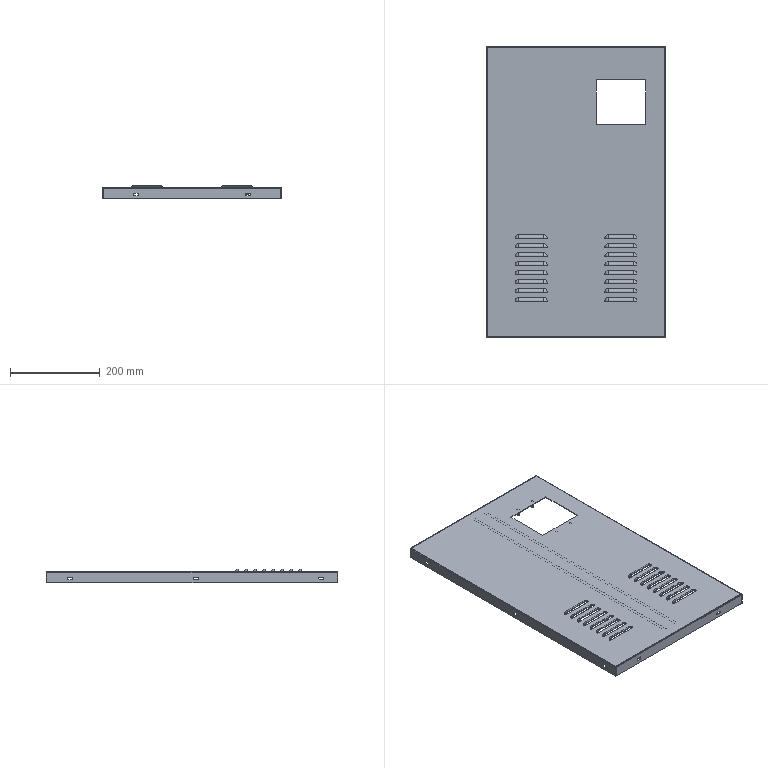Part | STEP file | FBDS-BJ-001 | 2 solids | 516 faces | box 398 x 648 x 31 mm | volume 500779 mm3 | cylinder 240 | plane 128 | torus 64 | sphere 64 | spline 20 | commonest cylinder face diameters 5 x128 6.5 x20 1 x16 4 x16 12 x16 15 x16